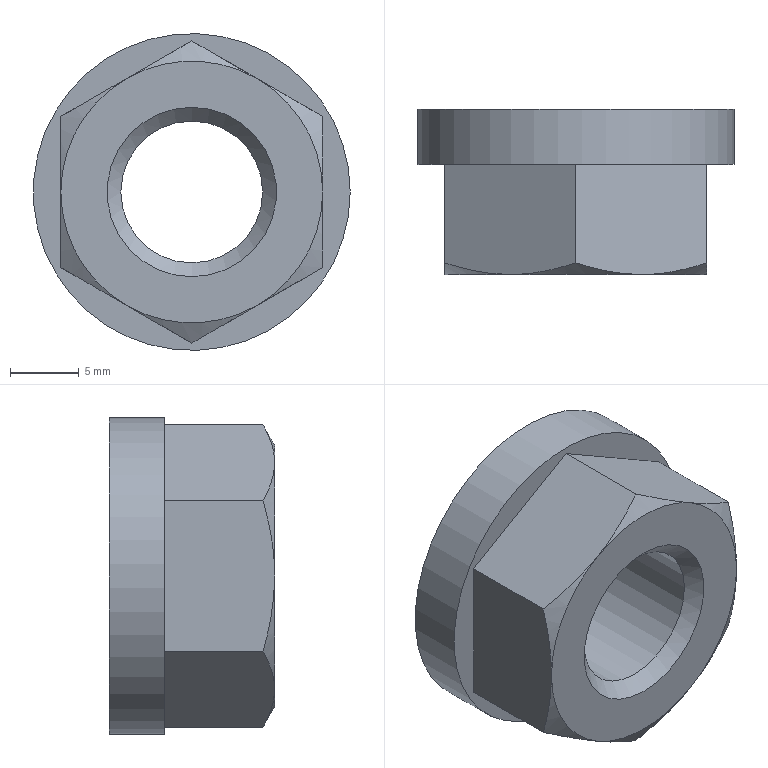Part | NX | features DATUM_CSYS 4, SKETCH 3, CHAMFER 2, EXTRUDE 2, HOLE PACKAGE 1, SIMPLE HOLE 1, SWP104 1, SYMBOLIC_THREAD 1 | 1 solid | 19 faces | box 23 x 12 x 23 mm | volume 3134 mm3 | plane 9 | cone 8 | cylinder 2 | commonest cylinder face diameters 10.3 x1 23 x1
STEP:
#1=CARTESIAN_POINT('',(-9.5,-7.151,-5.485));
#2=VERTEX_POINT('',#1);
#3=CARTESIAN_POINT('',(-9.5,0.,-5.485));
#4=VERTEX_POINT('',#3);
#5=CARTESIAN_POINT('',(-9.5,-8.,-5.485));
#6=DIRECTION('',(0.,1.,0.));
#7=VECTOR('',#6,1000.);
#8=LINE('',#5,#7);
#9=EDGE_CURVE('',#2,#4,#8,.T.);
#10=ORIENTED_EDGE('',*,*,#9,.F.);
#11=CARTESIAN_POINT('',(-9.5,-8.,0.));
#12=VERTEX_POINT('',#11);
#13=CARTESIAN_POINT('',(-9.5,-7.151,-5.485));
#14=CARTESIAN_POINT('',(-9.5,-7.667,-3.698));
#15=CARTESIAN_POINT('',(-9.5,-8.,-1.857));
#16=CARTESIAN_POINT('',(-9.5,-8.,0.));
#17=B_SPLINE_CURVE_WITH_KNOTS('',3,(#13,#14,#15,#16),.UNSPECIFIED.,.F.,.F.,(4,4),(0.01028,0.01583),.UNSPECIFIED.);
#18=EDGE_CURVE('',#2,#12,#17,.T.);
#19=ORIENTED_EDGE('',*,*,#18,.T.);
#20=CARTESIAN_POINT('',(-9.5,-7.151,5.485));
#21=VERTEX_POINT('',#20);
#22=CARTESIAN_POINT('',(-9.5,-8.,0.));
#23=CARTESIAN_POINT('',(-9.5,-8.,1.858));
#24=CARTESIAN_POINT('',(-9.5,-7.664,3.71));
#25=CARTESIAN_POINT('',(-9.5,-7.151,5.485));
#26=B_SPLINE_CURVE_WITH_KNOTS('',3,(#22,#23,#24,#25),.UNSPECIFIED.,.F.,.F.,(4,4),(0.01583,0.02139),.UNSPECIFIED.);
#27=EDGE_CURVE('',#12,#21,#26,.T.);
#28=ORIENTED_EDGE('',*,*,#27,.T.);
#29=CARTESIAN_POINT('',(-9.5,0.,5.485));
#30=VERTEX_POINT('',#29);
#31=CARTESIAN_POINT('',(-9.5,-8.,5.485));
#32=DIRECTION('',(0.,1.,0.));
#33=VECTOR('',#32,1000.);
#34=LINE('',#31,#33);
#35=EDGE_CURVE('',#21,#30,#34,.T.);
#36=ORIENTED_EDGE('',*,*,#35,.T.);
#37=CARTESIAN_POINT('',(-9.5,0.,5.485));
#38=DIRECTION('',(0.,0.,-1.));
#39=VECTOR('',#38,1000.);
#40=LINE('',#37,#39);
#41=EDGE_CURVE('',#30,#4,#40,.T.);
#42=ORIENTED_EDGE('',*,*,#41,.T.);
#43=EDGE_LOOP('',(#10,#19,#28,#36,#42));
#44=FACE_BOUND('',#43,.T.);
#45=CARTESIAN_POINT('',(-9.5,-8.,5.485));
#46=DIRECTION('',(1.,0.,0.));
#47=DIRECTION('',(0.,0.,-1.));
#48=AXIS2_PLACEMENT_3D('',#45,#46,#47);
#49=PLANE('',#48);
#50=ADVANCED_FACE('',(#44),#49,.F.);
#51=CARTESIAN_POINT('',(0.,-7.151,-10.97));
#52=VERTEX_POINT('',#51);
#53=CARTESIAN_POINT('',(0.,0.,-10.97));
#54=VERTEX_POINT('',#53);
#55=CARTESIAN_POINT('',(0.,-8.,-10.97));
#56=DIRECTION('',(0.,1.,0.));
#57=VECTOR('',#56,1000.);
#58=LINE('',#55,#57);
#59=EDGE_CURVE('',#52,#54,#58,.T.);
#60=ORIENTED_EDGE('',*,*,#59,.F.);
#61=CARTESIAN_POINT('',(-4.75,-8.,-8.227));
#62=VERTEX_POINT('',#61);
#63=CARTESIAN_POINT('',(0.,-7.151,-10.97));
#64=CARTESIAN_POINT('',(-1.554,-7.67,-10.072));
#65=CARTESIAN_POINT('',(-3.131,-8.,-9.162));
#66=CARTESIAN_POINT('',(-4.75,-8.,-8.227));
#67=B_SPLINE_CURVE_WITH_KNOTS('',3,(#63,#64,#65,#66),.UNSPECIFIED.,.F.,.F.,(4,4),(0.000000238,0.00555),.UNSPECIFIED.);
#68=EDGE_CURVE('',#52,#62,#67,.T.);
#69=ORIENTED_EDGE('',*,*,#68,.T.);
#70=CARTESIAN_POINT('',(-4.75,-8.,-8.227));
#71=CARTESIAN_POINT('',(-6.362,-8.,-7.296));
#72=CARTESIAN_POINT('',(-7.95,-7.668,-6.38));
#73=CARTESIAN_POINT('',(-9.5,-7.151,-5.485));
#74=B_SPLINE_CURVE_WITH_KNOTS('',3,(#70,#71,#72,#73),.UNSPECIFIED.,.F.,.F.,(4,4),(0.00555,0.01108),.UNSPECIFIED.);
#75=EDGE_CURVE('',#62,#2,#74,.T.);
#76=ORIENTED_EDGE('',*,*,#75,.T.);
#77=ORIENTED_EDGE('',*,*,#9,.T.);
#78=CARTESIAN_POINT('',(-9.5,0.,-5.485));
#79=DIRECTION('',(0.866,0.,-0.5));
#80=VECTOR('',#79,1000.);
#81=LINE('',#78,#80);
#82=EDGE_CURVE('',#4,#54,#81,.T.);
#83=ORIENTED_EDGE('',*,*,#82,.T.);
#84=EDGE_LOOP('',(#60,#69,#76,#77,#83));
#85=FACE_BOUND('',#84,.T.);
#86=CARTESIAN_POINT('',(-9.5,-8.,-5.485));
#87=DIRECTION('',(0.5,0.,0.866));
#88=DIRECTION('',(0.866,0.,-0.5));
#89=AXIS2_PLACEMENT_3D('',#86,#87,#88);
#90=PLANE('',#89);
#91=ADVANCED_FACE('',(#85),#90,.F.);
#92=CARTESIAN_POINT('',(9.5,-7.151,-5.485));
#93=VERTEX_POINT('',#92);
#94=CARTESIAN_POINT('',(9.5,0.,-5.485));
#95=VERTEX_POINT('',#94);
#96=CARTESIAN_POINT('',(9.5,-8.,-5.485));
#97=DIRECTION('',(0.,1.,0.));
#98=VECTOR('',#97,1000.);
#99=LINE('',#96,#98);
#100=EDGE_CURVE('',#93,#95,#99,.T.);
#101=ORIENTED_EDGE('',*,*,#100,.F.);
#102=CARTESIAN_POINT('',(4.75,-8.,-8.227));
#103=VERTEX_POINT('',#102);
#104=CARTESIAN_POINT('',(9.5,-7.151,-5.485));
#105=CARTESIAN_POINT('',(7.946,-7.67,-6.382));
#106=CARTESIAN_POINT('',(6.369,-8.,-7.293));
#107=CARTESIAN_POINT('',(4.75,-8.,-8.227));
#108=B_SPLINE_CURVE_WITH_KNOTS('',3,(#104,#105,#106,#107),.UNSPECIFIED.,.F.,.F.,(4,4),(0.000000238,0.00555),.UNSPECIFIED.);
#109=EDGE_CURVE('',#93,#103,#108,.T.);
#110=ORIENTED_EDGE('',*,*,#109,.T.);
#111=CARTESIAN_POINT('',(4.75,-8.,-8.227));
#112=CARTESIAN_POINT('',(3.138,-8.,-9.158));
#113=CARTESIAN_POINT('',(1.55,-7.668,-10.075));
#114=CARTESIAN_POINT('',(0.,-7.151,-10.97));
#115=B_SPLINE_CURVE_WITH_KNOTS('',3,(#111,#112,#113,#114),.UNSPECIFIED.,.F.,.F.,(4,4),(0.00555,0.01108),.UNSPECIFIED.);
#116=EDGE_CURVE('',#103,#52,#115,.T.);
#117=ORIENTED_EDGE('',*,*,#116,.T.);
#118=ORIENTED_EDGE('',*,*,#59,.T.);
#119=CARTESIAN_POINT('',(0.,0.,-10.97));
#120=DIRECTION('',(0.866,0.,0.5));
#121=VECTOR('',#120,1000.);
#122=LINE('',#119,#121);
#123=EDGE_CURVE('',#54,#95,#122,.T.);
#124=ORIENTED_EDGE('',*,*,#123,.T.);
#125=EDGE_LOOP('',(#101,#110,#117,#118,#124));
#126=FACE_BOUND('',#125,.T.);
#127=CARTESIAN_POINT('',(0.,-8.,-10.97));
#128=DIRECTION('',(-0.5,0.,0.866));
#129=DIRECTION('',(0.866,0.,0.5));
#130=AXIS2_PLACEMENT_3D('',#127,#128,#129);
#131=PLANE('',#130);
#132=ADVANCED_FACE('',(#126),#131,.F.);
#133=CARTESIAN_POINT('',(9.5,-7.151,5.485));
#134=VERTEX_POINT('',#133);
#135=CARTESIAN_POINT('',(9.5,0.,5.485));
#136=VERTEX_POINT('',#135);
#137=CARTESIAN_POINT('',(9.5,-8.,5.485));
#138=DIRECTION('',(0.,1.,0.));
#139=VECTOR('',#138,1000.);
#140=LINE('',#137,#139);
#141=EDGE_CURVE('',#134,#136,#140,.T.);
#142=ORIENTED_EDGE('',*,*,#141,.F.);
#143=CARTESIAN_POINT('',(9.5,-8.,0.));
#144=VERTEX_POINT('',#143);
#145=CARTESIAN_POINT('',(9.5,-8.,0.));
#146=CARTESIAN_POINT('',(9.5,-8.,1.858));
#147=CARTESIAN_POINT('',(9.5,-7.664,3.71));
#148=CARTESIAN_POINT('',(9.5,-7.151,5.485));
#149=B_SPLINE_CURVE_WITH_KNOTS('',3,(#145,#146,#147,#148),.UNSPECIFIED.,.F.,.F.,(4,4),(0.01583,0.02139),.UNSPECIFIED.);
#150=EDGE_CURVE('',#134,#144,#149,.F.);
#151=ORIENTED_EDGE('',*,*,#150,.T.);
#152=CARTESIAN_POINT('',(9.5,-7.151,-5.485));
#153=CARTESIAN_POINT('',(9.5,-7.667,-3.698));
#154=CARTESIAN_POINT('',(9.5,-8.,-1.857));
#155=CARTESIAN_POINT('',(9.5,-8.,0.));
#156=B_SPLINE_CURVE_WITH_KNOTS('',3,(#152,#153,#154,#155),.UNSPECIFIED.,.F.,.F.,(4,4),(0.01028,0.01583),.UNSPECIFIED.);
#157=EDGE_CURVE('',#144,#93,#156,.F.);
#158=ORIENTED_EDGE('',*,*,#157,.T.);
#159=ORIENTED_EDGE('',*,*,#100,.T.);
#160=CARTESIAN_POINT('',(9.5,0.,-5.485));
#161=DIRECTION('',(0.,0.,1.));
#162=VECTOR('',#161,1000.);
#163=LINE('',#160,#162);
#164=EDGE_CURVE('',#95,#136,#163,.T.);
#165=ORIENTED_EDGE('',*,*,#164,.T.);
#166=EDGE_LOOP('',(#142,#151,#158,#159,#165));
#167=FACE_BOUND('',#166,.T.);
#168=CARTESIAN_POINT('',(9.5,-8.,-5.485));
#169=DIRECTION('',(-1.,0.,0.));
#170=DIRECTION('',(0.,0.,1.));
#171=AXIS2_PLACEMENT_3D('',#168,#169,#170);
#172=PLANE('',#171);
#173=ADVANCED_FACE('',(#167),#172,.F.);
#174=CARTESIAN_POINT('',(0.,-7.151,10.97));
#175=VERTEX_POINT('',#174);
#176=CARTESIAN_POINT('',(0.,0.,10.97));
#177=VERTEX_POINT('',#176);
#178=CARTESIAN_POINT('',(0.,-8.,10.97));
#179=DIRECTION('',(0.,1.,0.));
#180=VECTOR('',#179,1000.);
#181=LINE('',#178,#180);
#182=EDGE_CURVE('',#175,#177,#181,.T.);
#183=ORIENTED_EDGE('',*,*,#182,.F.);
#184=CARTESIAN_POINT('',(4.75,-8.,8.227));
#185=VERTEX_POINT('',#184);
#186=CARTESIAN_POINT('',(0.,-7.151,10.97));
#187=CARTESIAN_POINT('',(1.554,-7.67,10.072));
#188=CARTESIAN_POINT('',(3.131,-8.,9.162));
#189=CARTESIAN_POINT('',(4.75,-8.,8.227));
#190=B_SPLINE_CURVE_WITH_KNOTS('',3,(#186,#187,#188,#189),.UNSPECIFIED.,.F.,.F.,(4,4),(0.000000238,0.00555),.UNSPECIFIED.);
#191=EDGE_CURVE('',#175,#185,#190,.T.);
#192=ORIENTED_EDGE('',*,*,#191,.T.);
#193=CARTESIAN_POINT('',(4.75,-8.,8.227));
#194=CARTESIAN_POINT('',(6.362,-8.,7.296));
#195=CARTESIAN_POINT('',(7.95,-7.668,6.38));
#196=CARTESIAN_POINT('',(9.5,-7.151,5.485));
#197=B_SPLINE_CURVE_WITH_KNOTS('',3,(#193,#194,#195,#196),.UNSPECIFIED.,.F.,.F.,(4,4),(0.00555,0.01108),.UNSPECIFIED.);
#198=EDGE_CURVE('',#185,#134,#197,.T.);
#199=ORIENTED_EDGE('',*,*,#198,.T.);
#200=ORIENTED_EDGE('',*,*,#141,.T.);
#201=CARTESIAN_POINT('',(9.5,0.,5.485));
#202=DIRECTION('',(-0.866,0.,0.5));
#203=VECTOR('',#202,1000.);
#204=LINE('',#201,#203);
#205=EDGE_CURVE('',#136,#177,#204,.T.);
#206=ORIENTED_EDGE('',*,*,#205,.T.);
#207=EDGE_LOOP('',(#183,#192,#199,#200,#206));
#208=FACE_BOUND('',#207,.T.);
#209=CARTESIAN_POINT('',(9.5,-8.,5.485));
#210=DIRECTION('',(-0.5,0.,-0.866));
#211=DIRECTION('',(-0.866,0.,0.5));
#212=AXIS2_PLACEMENT_3D('',#209,#210,#211);
#213=PLANE('',#212);
#214=ADVANCED_FACE('',(#208),#213,.F.);
#215=ORIENTED_EDGE('',*,*,#35,.F.);
#216=CARTESIAN_POINT('',(-4.75,-8.,8.227));
#217=VERTEX_POINT('',#216);
#218=CARTESIAN_POINT('',(-9.5,-7.151,5.485));
#219=CARTESIAN_POINT('',(-7.946,-7.67,6.382));
#220=CARTESIAN_POINT('',(-6.369,-8.,7.293));
#221=CARTESIAN_POINT('',(-4.75,-8.,8.227));
#222=B_SPLINE_CURVE_WITH_KNOTS('',3,(#218,#219,#220,#221),.UNSPECIFIED.,.F.,.F.,(4,4),(0.000000238,0.00555),.UNSPECIFIED.);
#223=EDGE_CURVE('',#21,#217,#222,.T.);
#224=ORIENTED_EDGE('',*,*,#223,.T.);
#225=CARTESIAN_POINT('',(-4.75,-8.,8.227));
#226=CARTESIAN_POINT('',(-3.138,-8.,9.158));
#227=CARTESIAN_POINT('',(-1.55,-7.668,10.075));
#228=CARTESIAN_POINT('',(0.,-7.151,10.97));
#229=B_SPLINE_CURVE_WITH_KNOTS('',3,(#225,#226,#227,#228),.UNSPECIFIED.,.F.,.F.,(4,4),(0.00555,0.01108),.UNSPECIFIED.);
#230=EDGE_CURVE('',#217,#175,#229,.T.);
#231=ORIENTED_EDGE('',*,*,#230,.T.);
#232=ORIENTED_EDGE('',*,*,#182,.T.);
#233=CARTESIAN_POINT('',(0.,0.,10.97));
#234=DIRECTION('',(-0.866,0.,-0.5));
#235=VECTOR('',#234,1000.);
#236=LINE('',#233,#235);
#237=EDGE_CURVE('',#177,#30,#236,.T.);
#238=ORIENTED_EDGE('',*,*,#237,.T.);
#239=EDGE_LOOP('',(#215,#224,#231,#232,#238));
#240=FACE_BOUND('',#239,.T.);
#241=CARTESIAN_POINT('',(0.,-8.,10.97));
#242=DIRECTION('',(0.5,0.,-0.866));
#243=DIRECTION('',(-0.866,0.,-0.5));
#244=AXIS2_PLACEMENT_3D('',#241,#242,#243);
#245=PLANE('',#244);
#246=ADVANCED_FACE('',(#240),#245,.F.);
#247=CARTESIAN_POINT('',(11.5,0.,0.));
#248=VERTEX_POINT('',#247);
#249=CARTESIAN_POINT('',(0.,0.,0.));
#250=DIRECTION('',(0.,-1.,0.));
#251=DIRECTION('',(1.,0.,0.));
#252=AXIS2_PLACEMENT_3D('',#249,#250,#251);
#253=CIRCLE('',#252,11.5);
#254=EDGE_CURVE('',#248,#248,#253,.T.);
#255=ORIENTED_EDGE('',*,*,#254,.T.);
#256=EDGE_LOOP('',(#255));
#257=FACE_BOUND('',#256,.T.);
#258=ORIENTED_EDGE('',*,*,#41,.F.);
#259=ORIENTED_EDGE('',*,*,#237,.F.);
#260=ORIENTED_EDGE('',*,*,#205,.F.);
#261=ORIENTED_EDGE('',*,*,#164,.F.);
#262=ORIENTED_EDGE('',*,*,#123,.F.);
#263=ORIENTED_EDGE('',*,*,#82,.F.);
#264=EDGE_LOOP('',(#258,#259,#260,#261,#262,#263));
#265=FACE_BOUND('',#264,.T.);
#266=CARTESIAN_POINT('',(0.,0.,0.));
#267=DIRECTION('',(0.,-1.,0.));
#268=DIRECTION('',(0.,0.,-1.));
#269=AXIS2_PLACEMENT_3D('',#266,#267,#268);
#270=PLANE('',#269);
#271=ADVANCED_FACE('',(#257,#265),#270,.T.);
#272=CARTESIAN_POINT('',(11.5,4.,0.));
#273=VERTEX_POINT('',#272);
#274=CARTESIAN_POINT('',(0.,4.,0.));
#275=DIRECTION('',(0.,-1.,0.));
#276=DIRECTION('',(1.,0.,0.));
#277=AXIS2_PLACEMENT_3D('',#274,#275,#276);
#278=CIRCLE('',#277,11.5);
#279=EDGE_CURVE('',#273,#273,#278,.T.);
#280=ORIENTED_EDGE('',*,*,#279,.T.);
#281=EDGE_LOOP('',(#280));
#282=FACE_BOUND('',#281,.T.);
#283=ORIENTED_EDGE('',*,*,#254,.F.);
#284=EDGE_LOOP('',(#283));
#285=FACE_BOUND('',#284,.T.);
#286=CARTESIAN_POINT('',(0.,4.,0.));
#287=DIRECTION('',(0.,-1.,0.));
#288=DIRECTION('',(0.,0.,-1.));
#289=AXIS2_PLACEMENT_3D('',#286,#287,#288);
#290=CYLINDRICAL_SURFACE('',#289,11.5);
#291=ADVANCED_FACE('',(#282,#285),#290,.T.);
#292=CARTESIAN_POINT('',(0.,4.,-5.65));
#293=VERTEX_POINT('',#292);
#294=CARTESIAN_POINT('',(0.,4.,0.));
#295=DIRECTION('',(0.,-1.,0.));
#296=DIRECTION('',(0.,0.,-1.));
#297=AXIS2_PLACEMENT_3D('',#294,#295,#296);
#298=CIRCLE('',#297,5.65);
#299=EDGE_CURVE('',#293,#293,#298,.T.);
#300=ORIENTED_EDGE('',*,*,#299,.T.);
#301=EDGE_LOOP('',(#300));
#302=FACE_BOUND('',#301,.T.);
#303=ORIENTED_EDGE('',*,*,#279,.F.);
#304=EDGE_LOOP('',(#303));
#305=FACE_BOUND('',#304,.T.);
#306=CARTESIAN_POINT('',(0.,4.,0.));
#307=DIRECTION('',(0.,-1.,0.));
#308=DIRECTION('',(0.,0.,-1.));
#309=AXIS2_PLACEMENT_3D('',#306,#307,#308);
#310=PLANE('',#309);
#311=ADVANCED_FACE('',(#302,#305),#310,.F.);
#312=ORIENTED_EDGE('',*,*,#230,.F.);
#313=CARTESIAN_POINT('',(0.,-8.,0.));
#314=DIRECTION('',(0.,-1.,0.));
#315=DIRECTION('',(0.,0.,-1.));
#316=AXIS2_PLACEMENT_3D('',#313,#314,#315);
#317=CIRCLE('',#316,9.5);
#318=EDGE_CURVE('',#185,#217,#317,.T.);
#319=ORIENTED_EDGE('',*,*,#318,.F.);
#320=ORIENTED_EDGE('',*,*,#191,.F.);
#321=EDGE_LOOP('',(#312,#319,#320));
#322=FACE_BOUND('',#321,.T.);
#323=CARTESIAN_POINT('',(0.,-4.005,0.));
#324=DIRECTION('',(0.,1.,0.));
#325=DIRECTION('',(0.,0.,1.));
#326=AXIS2_PLACEMENT_3D('',#323,#324,#325);
#327=CONICAL_SURFACE('',#326,16.419,1.047);
#328=ADVANCED_FACE('',(#322),#327,.T.);
#329=CARTESIAN_POINT('',(0.,-8.,0.));
#330=DIRECTION('',(0.,-1.,0.));
#331=DIRECTION('',(0.,0.,-1.));
#332=AXIS2_PLACEMENT_3D('',#329,#330,#331);
#333=CIRCLE('',#332,9.5);
#334=EDGE_CURVE('',#217,#12,#333,.T.);
#335=ORIENTED_EDGE('',*,*,#334,.F.);
#336=ORIENTED_EDGE('',*,*,#223,.F.);
#337=ORIENTED_EDGE('',*,*,#27,.F.);
#338=EDGE_LOOP('',(#335,#336,#337));
#339=FACE_BOUND('',#338,.T.);
#340=CARTESIAN_POINT('',(0.,-4.005,0.));
#341=DIRECTION('',(0.,1.,0.));
#342=DIRECTION('',(0.,0.,1.));
#343=AXIS2_PLACEMENT_3D('',#340,#341,#342);
#344=CONICAL_SURFACE('',#343,16.419,1.047);
#345=ADVANCED_FACE('',(#339),#344,.T.);
#346=ORIENTED_EDGE('',*,*,#198,.F.);
#347=CARTESIAN_POINT('',(0.,-8.,0.));
#348=DIRECTION('',(0.,-1.,0.));
#349=DIRECTION('',(0.,0.,-1.));
#350=AXIS2_PLACEMENT_3D('',#347,#348,#349);
#351=CIRCLE('',#350,9.5);
#352=EDGE_CURVE('',#144,#185,#351,.T.);
#353=ORIENTED_EDGE('',*,*,#352,.F.);
#354=ORIENTED_EDGE('',*,*,#150,.F.);
#355=EDGE_LOOP('',(#346,#353,#354));
#356=FACE_BOUND('',#355,.T.);
#357=CARTESIAN_POINT('',(0.,-4.005,0.));
#358=DIRECTION('',(0.,1.,0.));
#359=DIRECTION('',(0.,0.,1.));
#360=AXIS2_PLACEMENT_3D('',#357,#358,#359);
#361=CONICAL_SURFACE('',#360,16.419,1.047);
#362=ADVANCED_FACE('',(#356),#361,.T.);
#363=ORIENTED_EDGE('',*,*,#157,.F.);
#364=CARTESIAN_POINT('',(0.,-8.,0.));
#365=DIRECTION('',(0.,-1.,0.));
#366=DIRECTION('',(0.,0.,-1.));
#367=AXIS2_PLACEMENT_3D('',#364,#365,#366);
#368=CIRCLE('',#367,9.5);
#369=EDGE_CURVE('',#103,#144,#368,.T.);
#370=ORIENTED_EDGE('',*,*,#369,.F.);
#371=ORIENTED_EDGE('',*,*,#109,.F.);
#372=EDGE_LOOP('',(#363,#370,#371));
#373=FACE_BOUND('',#372,.T.);
#374=CARTESIAN_POINT('',(0.,-4.005,0.));
#375=DIRECTION('',(0.,1.,0.));
#376=DIRECTION('',(0.,0.,1.));
#377=AXIS2_PLACEMENT_3D('',#374,#375,#376);
#378=CONICAL_SURFACE('',#377,16.419,1.047);
#379=ADVANCED_FACE('',(#373),#378,.T.);
#380=CARTESIAN_POINT('',(0.,-8.,0.));
#381=DIRECTION('',(0.,-1.,0.));
#382=DIRECTION('',(0.,0.,-1.));
#383=AXIS2_PLACEMENT_3D('',#380,#381,#382);
#384=CIRCLE('',#383,9.5);
#385=EDGE_CURVE('',#62,#103,#384,.T.);
#386=ORIENTED_EDGE('',*,*,#385,.F.);
#387=ORIENTED_EDGE('',*,*,#68,.F.);
#388=ORIENTED_EDGE('',*,*,#116,.F.);
#389=EDGE_LOOP('',(#386,#387,#388));
#390=FACE_BOUND('',#389,.T.);
#391=CARTESIAN_POINT('',(0.,-4.005,0.));
#392=DIRECTION('',(0.,1.,0.));
#393=DIRECTION('',(0.,0.,1.));
#394=AXIS2_PLACEMENT_3D('',#391,#392,#393);
#395=CONICAL_SURFACE('',#394,16.419,1.047);
#396=ADVANCED_FACE('',(#390),#395,.T.);
#397=CARTESIAN_POINT('',(0.,-8.,0.));
#398=DIRECTION('',(0.,-1.,0.));
#399=DIRECTION('',(0.,0.,-1.));
#400=AXIS2_PLACEMENT_3D('',#397,#398,#399);
#401=CIRCLE('',#400,9.5);
#402=EDGE_CURVE('',#12,#62,#401,.T.);
#403=ORIENTED_EDGE('',*,*,#402,.F.);
#404=ORIENTED_EDGE('',*,*,#18,.F.);
#405=ORIENTED_EDGE('',*,*,#75,.F.);
#406=EDGE_LOOP('',(#403,#404,#405));
#407=FACE_BOUND('',#406,.T.);
#408=CARTESIAN_POINT('',(0.,-4.005,0.));
#409=DIRECTION('',(0.,1.,0.));
#410=DIRECTION('',(0.,0.,1.));
#411=AXIS2_PLACEMENT_3D('',#408,#409,#410);
#412=CONICAL_SURFACE('',#411,16.419,1.047);
#413=ADVANCED_FACE('',(#407),#412,.T.);
#414=CARTESIAN_POINT('',(0.,-8.,-6.15));
#415=VERTEX_POINT('',#414);
#416=CARTESIAN_POINT('',(0.,-8.,0.));
#417=DIRECTION('',(0.,-1.,0.));
#418=DIRECTION('',(0.,0.,-1.));
#419=AXIS2_PLACEMENT_3D('',#416,#417,#418);
#420=CIRCLE('',#419,6.15);
#421=EDGE_CURVE('',#415,#415,#420,.F.);
#422=ORIENTED_EDGE('',*,*,#421,.T.);
#423=EDGE_LOOP('',(#422));
#424=FACE_BOUND('',#423,.T.);
#425=ORIENTED_EDGE('',*,*,#385,.T.);
#426=ORIENTED_EDGE('',*,*,#369,.T.);
#427=ORIENTED_EDGE('',*,*,#352,.T.);
#428=ORIENTED_EDGE('',*,*,#318,.T.);
#429=ORIENTED_EDGE('',*,*,#334,.T.);
#430=ORIENTED_EDGE('',*,*,#402,.T.);
#431=EDGE_LOOP('',(#425,#426,#427,#428,#429,#430));
#432=FACE_BOUND('',#431,.T.);
#433=CARTESIAN_POINT('',(0.,-8.,0.));
#434=DIRECTION('',(0.,-1.,0.));
#435=DIRECTION('',(0.,0.,-1.));
#436=AXIS2_PLACEMENT_3D('',#433,#434,#435);
#437=PLANE('',#436);
#438=ADVANCED_FACE('',(#424,#432),#437,.T.);
#439=CARTESIAN_POINT('',(0.,3.5,-5.15));
#440=VERTEX_POINT('',#439);
#441=CARTESIAN_POINT('',(0.,3.5,0.));
#442=DIRECTION('',(0.,-1.,0.));
#443=DIRECTION('',(0.,0.,-1.));
#444=AXIS2_PLACEMENT_3D('',#441,#442,#443);
#445=CIRCLE('',#444,5.15);
#446=EDGE_CURVE('',#440,#440,#445,.F.);
#447=ORIENTED_EDGE('',*,*,#446,.T.);
#448=EDGE_LOOP('',(#447));
#449=FACE_BOUND('',#448,.T.);
#450=CARTESIAN_POINT('',(0.,-7.,-5.15));
#451=VERTEX_POINT('',#450);
#452=CARTESIAN_POINT('',(0.,-7.,0.));
#453=DIRECTION('',(0.,-1.,0.));
#454=DIRECTION('',(0.,0.,-1.));
#455=AXIS2_PLACEMENT_3D('',#452,#453,#454);
#456=CIRCLE('',#455,5.15);
#457=EDGE_CURVE('',#451,#451,#456,.T.);
#458=ORIENTED_EDGE('',*,*,#457,.T.);
#459=EDGE_LOOP('',(#458));
#460=FACE_BOUND('',#459,.T.);
#461=CARTESIAN_POINT('',(0.,-8.,0.));
#462=DIRECTION('',(0.,1.,0.));
#463=DIRECTION('',(0.,0.,1.));
#464=AXIS2_PLACEMENT_3D('',#461,#462,#463);
#465=CYLINDRICAL_SURFACE('',#464,5.15);
#466=ADVANCED_FACE('',(#449,#460),#465,.F.);
#467=ORIENTED_EDGE('',*,*,#457,.F.);
#468=EDGE_LOOP('',(#467));
#469=FACE_BOUND('',#468,.T.);
#470=ORIENTED_EDGE('',*,*,#421,.F.);
#471=EDGE_LOOP('',(#470));
#472=FACE_BOUND('',#471,.T.);
#473=CARTESIAN_POINT('',(0.,-8.,0.));
#474=DIRECTION('',(0.,-1.,0.));
#475=DIRECTION('',(0.,0.,-1.));
#476=AXIS2_PLACEMENT_3D('',#473,#474,#475);
#477=CONICAL_SURFACE('',#476,6.15,0.7854);
#478=ADVANCED_FACE('',(#469,#472),#477,.F.);
#479=ORIENTED_EDGE('',*,*,#446,.F.);
#480=EDGE_LOOP('',(#479));
#481=FACE_BOUND('',#480,.T.);
#482=ORIENTED_EDGE('',*,*,#299,.F.);
#483=EDGE_LOOP('',(#482));
#484=FACE_BOUND('',#483,.T.);
#485=CARTESIAN_POINT('',(0.,4.,0.));
#486=DIRECTION('',(0.,1.,0.));
#487=DIRECTION('',(0.,0.,1.));
#488=AXIS2_PLACEMENT_3D('',#485,#486,#487);
#489=CONICAL_SURFACE('',#488,5.65,0.7854);
#490=ADVANCED_FACE('',(#481,#484),#489,.F.);
#491=CLOSED_SHELL('',(#50,#91,#132,#173,#214,#246,#271,#291,#311,#328,#345,#362,#379,#396,#413,#438,#466,#478,#490));
#492=MANIFOLD_SOLID_BREP('',#491);
#493=(LENGTH_UNIT()NAMED_UNIT(*)SI_UNIT(.MILLI.,.METRE.));
#494=UNCERTAINTY_MEASURE_WITH_UNIT(LENGTH_MEASURE(0.0508),#493,'','');
#495=(NAMED_UNIT(*)PLANE_ANGLE_UNIT()SI_UNIT($,.RADIAN.));
#496=(NAMED_UNIT(*)SI_UNIT($,.STERADIAN.)SOLID_ANGLE_UNIT());
#497=(GEOMETRIC_REPRESENTATION_CONTEXT(3)GLOBAL_UNCERTAINTY_ASSIGNED_CONTEXT((#494))GLOBAL_UNIT_ASSIGNED_CONTEXT((#493,#495,#496))REPRESENTATION_CONTEXT('',''));
#498=ADVANCED_BREP_SHAPE_REPRESENTATION('',(#492),#497);